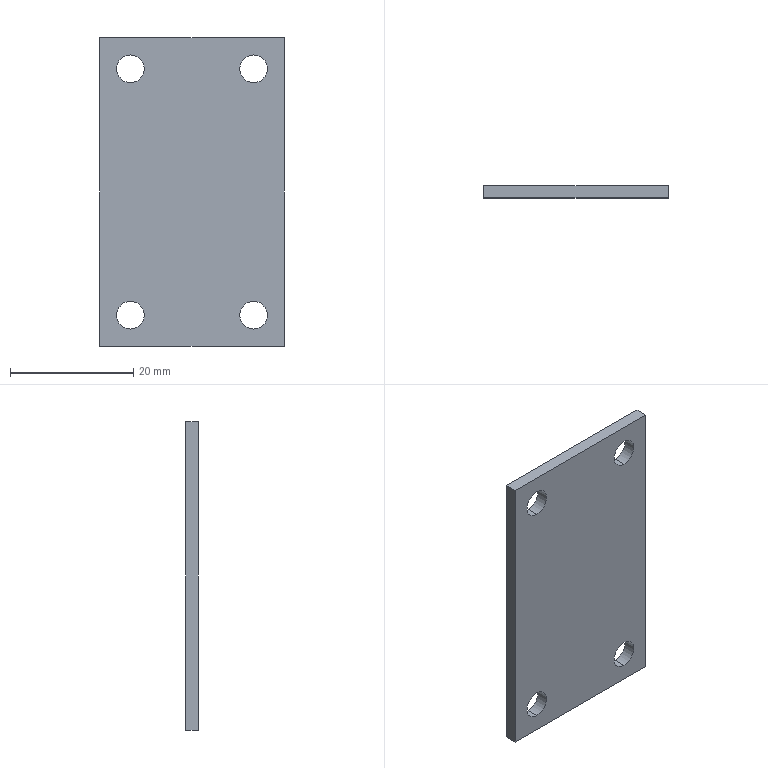Part | STEP file | 0243_204_Push_Plate | 1 solid | 14 faces | box 30 x 2 x 50 mm | volume 2873 mm3 | cylinder 8 | plane 6 | commonest cylinder face diameters 4.5 x8
STEP:
#1=CARTESIAN_POINT('',(0.,0.,0.));
#2=DIRECTION('',(0.,0.,1.));
#3=DIRECTION('',(1.,0.,0.));
#4=AXIS2_PLACEMENT_3D('',#1,#2,#3);
#5=CARTESIAN_POINT('',(-25.,0.,22.25));
#6=VERTEX_POINT('',#5);
#7=CARTESIAN_POINT('',(-25.,2.,22.25));
#8=VERTEX_POINT('',#7);
#9=CARTESIAN_POINT('',(-25.,2.,22.25));
#10=DIRECTION('',(0.,1.,0.));
#11=VECTOR('',#10,1.);
#12=LINE('',#9,#11);
#13=CARTESIAN_POINT('',(-25.,2.,20.));
#14=DIRECTION('',(0.,1.,0.));
#15=DIRECTION('',(0.,0.,1.));
#16=AXIS2_PLACEMENT_3D('',#13,#14,#15);
#17=CYLINDRICAL_SURFACE('',#16,2.25);
#18=CARTESIAN_POINT('',(6.283,0.));
#19=DIRECTION('',(0.,1.));
#20=VECTOR('',#19,1.);
#21=LINE('',#18,#20);
#22=(GEOMETRIC_REPRESENTATION_CONTEXT(2)PARAMETRIC_REPRESENTATION_CONTEXT()REPRESENTATION_CONTEXT('',''));
#23=DEFINITIONAL_REPRESENTATION('',(#21),#22);
#24=PCURVE('',#17,#23);
#25=CARTESIAN_POINT('',(-25.,2.,20.));
#26=DIRECTION('',(0.,1.,0.));
#27=DIRECTION('',(0.,0.,1.));
#28=AXIS2_PLACEMENT_3D('',#25,#26,#27);
#29=CYLINDRICAL_SURFACE('',#28,2.25);
#30=CARTESIAN_POINT('',(0.,0.));
#31=DIRECTION('',(0.,1.));
#32=VECTOR('',#31,1.);
#33=LINE('',#30,#32);
#34=(GEOMETRIC_REPRESENTATION_CONTEXT(2)PARAMETRIC_REPRESENTATION_CONTEXT()REPRESENTATION_CONTEXT('',''));
#35=DEFINITIONAL_REPRESENTATION('',(#33),#34);
#36=PCURVE('',#29,#35);
#37=SURFACE_CURVE('',#12,(#24,#36),.PCURVE_S1.);
#38=EDGE_CURVE('',#6,#8,#37,.T.);
#39=ORIENTED_EDGE('',*,*,#38,.T.);
#40=CARTESIAN_POINT('',(-25.,2.,17.75));
#41=VERTEX_POINT('',#40);
#42=CARTESIAN_POINT('',(-25.,2.,20.));
#43=DIRECTION('',(0.,1.,0.));
#44=DIRECTION('',(0.,0.,1.));
#45=AXIS2_PLACEMENT_3D('',#42,#43,#44);
#46=CIRCLE('',#45,2.25);
#47=CARTESIAN_POINT('',(0.,0.));
#48=DIRECTION('',(1.,0.));
#49=VECTOR('',#48,1.);
#50=LINE('',#47,#49);
#51=(GEOMETRIC_REPRESENTATION_CONTEXT(2)PARAMETRIC_REPRESENTATION_CONTEXT()REPRESENTATION_CONTEXT('',''));
#52=DEFINITIONAL_REPRESENTATION('',(#50),#51);
#53=PCURVE('',#17,#52);
#54=CARTESIAN_POINT('',(-30.,2.,25.));
#55=DIRECTION('',(0.,-1.,0.));
#56=DIRECTION('',(0.,0.,-1.));
#57=AXIS2_PLACEMENT_3D('',#54,#55,#56);
#58=PLANE('',#57);
#59=CARTESIAN_POINT('',(2.75,5.));
#60=CARTESIAN_POINT('',(2.75,8.897));
#61=CARTESIAN_POINT('',(6.125,6.949));
#62=CARTESIAN_POINT('',(9.5,5.));
#63=CARTESIAN_POINT('',(6.125,3.051));
#64=CARTESIAN_POINT('',(2.75,1.103));
#65=CARTESIAN_POINT('',(2.75,5.));
#66=(BOUNDED_CURVE()B_SPLINE_CURVE(2,(#59,#60,#61,#62,#63,#64,#65),.UNSPECIFIED.,.T.,.F.)B_SPLINE_CURVE_WITH_KNOTS((1,2,2,2,2,1),(-2.094,0.,2.094,4.189,6.283,8.378),.UNSPECIFIED.)CURVE()GEOMETRIC_REPRESENTATION_ITEM()RATIONAL_B_SPLINE_CURVE((1.,0.5,1.,0.5,1.,0.5,1.))REPRESENTATION_ITEM(''));
#67=(GEOMETRIC_REPRESENTATION_CONTEXT(2)PARAMETRIC_REPRESENTATION_CONTEXT()REPRESENTATION_CONTEXT('',''));
#68=DEFINITIONAL_REPRESENTATION('',(#66),#67);
#69=PCURVE('',#58,#68);
#70=SURFACE_CURVE('',#46,(#53,#69),.PCURVE_S1.);
#71=EDGE_CURVE('',#41,#8,#70,.T.);
#72=ORIENTED_EDGE('',*,*,#71,.F.);
#73=CARTESIAN_POINT('',(-25.,0.,17.75));
#74=VERTEX_POINT('',#73);
#75=CARTESIAN_POINT('',(-25.,2.,17.75));
#76=DIRECTION('',(0.,1.,0.));
#77=VECTOR('',#76,1.);
#78=LINE('',#75,#77);
#79=CARTESIAN_POINT('',(3.142,0.));
#80=DIRECTION('',(0.,1.));
#81=VECTOR('',#80,1.);
#82=LINE('',#79,#81);
#83=(GEOMETRIC_REPRESENTATION_CONTEXT(2)PARAMETRIC_REPRESENTATION_CONTEXT()REPRESENTATION_CONTEXT('',''));
#84=DEFINITIONAL_REPRESENTATION('',(#82),#83);
#85=PCURVE('',#17,#84);
#86=CARTESIAN_POINT('',(3.142,0.));
#87=DIRECTION('',(0.,1.));
#88=VECTOR('',#87,1.);
#89=LINE('',#86,#88);
#90=(GEOMETRIC_REPRESENTATION_CONTEXT(2)PARAMETRIC_REPRESENTATION_CONTEXT()REPRESENTATION_CONTEXT('',''));
#91=DEFINITIONAL_REPRESENTATION('',(#89),#90);
#92=PCURVE('',#29,#91);
#93=SURFACE_CURVE('',#78,(#85,#92),.PCURVE_S1.);
#94=EDGE_CURVE('',#74,#41,#93,.T.);
#95=ORIENTED_EDGE('',*,*,#94,.F.);
#96=CARTESIAN_POINT('',(-25.,0.,20.));
#97=DIRECTION('',(0.,1.,0.));
#98=DIRECTION('',(0.,0.,1.));
#99=AXIS2_PLACEMENT_3D('',#96,#97,#98);
#100=CIRCLE('',#99,2.25);
#101=CARTESIAN_POINT('',(0.,-2.));
#102=DIRECTION('',(1.,0.));
#103=VECTOR('',#102,1.);
#104=LINE('',#101,#103);
#105=(GEOMETRIC_REPRESENTATION_CONTEXT(2)PARAMETRIC_REPRESENTATION_CONTEXT()REPRESENTATION_CONTEXT('',''));
#106=DEFINITIONAL_REPRESENTATION('',(#104),#105);
#107=PCURVE('',#17,#106);
#108=CARTESIAN_POINT('',(-30.,0.,25.));
#109=DIRECTION('',(0.,-1.,0.));
#110=DIRECTION('',(0.,0.,-1.));
#111=AXIS2_PLACEMENT_3D('',#108,#109,#110);
#112=PLANE('',#111);
#113=CARTESIAN_POINT('',(2.75,5.));
#114=CARTESIAN_POINT('',(2.75,8.897));
#115=CARTESIAN_POINT('',(6.125,6.949));
#116=CARTESIAN_POINT('',(9.5,5.));
#117=CARTESIAN_POINT('',(6.125,3.051));
#118=CARTESIAN_POINT('',(2.75,1.103));
#119=CARTESIAN_POINT('',(2.75,5.));
#120=(BOUNDED_CURVE()B_SPLINE_CURVE(2,(#113,#114,#115,#116,#117,#118,#119),.UNSPECIFIED.,.T.,.F.)B_SPLINE_CURVE_WITH_KNOTS((1,2,2,2,2,1),(-2.094,0.,2.094,4.189,6.283,8.378),.UNSPECIFIED.)CURVE()GEOMETRIC_REPRESENTATION_ITEM()RATIONAL_B_SPLINE_CURVE((1.,0.5,1.,0.5,1.,0.5,1.))REPRESENTATION_ITEM(''));
#121=(GEOMETRIC_REPRESENTATION_CONTEXT(2)PARAMETRIC_REPRESENTATION_CONTEXT()REPRESENTATION_CONTEXT('',''));
#122=DEFINITIONAL_REPRESENTATION('',(#120),#121);
#123=PCURVE('',#112,#122);
#124=SURFACE_CURVE('',#100,(#107,#123),.PCURVE_S1.);
#125=EDGE_CURVE('',#74,#6,#124,.T.);
#126=ORIENTED_EDGE('',*,*,#125,.T.);
#127=EDGE_LOOP('',(#39,#72,#95,#126));
#128=FACE_BOUND('',#127,.F.);
#129=ADVANCED_FACE('',(#128),#17,.F.);
#130=CARTESIAN_POINT('',(-25.,0.,-17.75));
#131=VERTEX_POINT('',#130);
#132=CARTESIAN_POINT('',(-25.,2.,-17.75));
#133=VERTEX_POINT('',#132);
#134=CARTESIAN_POINT('',(-25.,2.,-17.75));
#135=DIRECTION('',(0.,1.,0.));
#136=VECTOR('',#135,1.);
#137=LINE('',#134,#136);
#138=CARTESIAN_POINT('',(-25.,2.,-20.));
#139=DIRECTION('',(0.,1.,0.));
#140=DIRECTION('',(0.,0.,1.));
#141=AXIS2_PLACEMENT_3D('',#138,#139,#140);
#142=CYLINDRICAL_SURFACE('',#141,2.25);
#143=CARTESIAN_POINT('',(6.283,0.));
#144=DIRECTION('',(0.,1.));
#145=VECTOR('',#144,1.);
#146=LINE('',#143,#145);
#147=(GEOMETRIC_REPRESENTATION_CONTEXT(2)PARAMETRIC_REPRESENTATION_CONTEXT()REPRESENTATION_CONTEXT('',''));
#148=DEFINITIONAL_REPRESENTATION('',(#146),#147);
#149=PCURVE('',#142,#148);
#150=CARTESIAN_POINT('',(-25.,2.,-20.));
#151=DIRECTION('',(0.,1.,0.));
#152=DIRECTION('',(0.,0.,1.));
#153=AXIS2_PLACEMENT_3D('',#150,#151,#152);
#154=CYLINDRICAL_SURFACE('',#153,2.25);
#155=CARTESIAN_POINT('',(0.,0.));
#156=DIRECTION('',(0.,1.));
#157=VECTOR('',#156,1.);
#158=LINE('',#155,#157);
#159=(GEOMETRIC_REPRESENTATION_CONTEXT(2)PARAMETRIC_REPRESENTATION_CONTEXT()REPRESENTATION_CONTEXT('',''));
#160=DEFINITIONAL_REPRESENTATION('',(#158),#159);
#161=PCURVE('',#154,#160);
#162=SURFACE_CURVE('',#137,(#149,#161),.PCURVE_S1.);
#163=EDGE_CURVE('',#131,#133,#162,.T.);
#164=ORIENTED_EDGE('',*,*,#163,.T.);
#165=CARTESIAN_POINT('',(-25.,2.,-22.25));
#166=VERTEX_POINT('',#165);
#167=CARTESIAN_POINT('',(-25.,2.,-20.));
#168=DIRECTION('',(0.,1.,0.));
#169=DIRECTION('',(0.,0.,1.));
#170=AXIS2_PLACEMENT_3D('',#167,#168,#169);
#171=CIRCLE('',#170,2.25);
#172=CARTESIAN_POINT('',(0.,0.));
#173=DIRECTION('',(1.,0.));
#174=VECTOR('',#173,1.);
#175=LINE('',#172,#174);
#176=(GEOMETRIC_REPRESENTATION_CONTEXT(2)PARAMETRIC_REPRESENTATION_CONTEXT()REPRESENTATION_CONTEXT('',''));
#177=DEFINITIONAL_REPRESENTATION('',(#175),#176);
#178=PCURVE('',#142,#177);
#179=CARTESIAN_POINT('',(42.75,5.));
#180=CARTESIAN_POINT('',(42.75,8.897));
#181=CARTESIAN_POINT('',(46.125,6.949));
#182=CARTESIAN_POINT('',(49.5,5.));
#183=CARTESIAN_POINT('',(46.125,3.051));
#184=CARTESIAN_POINT('',(42.75,1.103));
#185=CARTESIAN_POINT('',(42.75,5.));
#186=(BOUNDED_CURVE()B_SPLINE_CURVE(2,(#179,#180,#181,#182,#183,#184,#185),.UNSPECIFIED.,.T.,.F.)B_SPLINE_CURVE_WITH_KNOTS((1,2,2,2,2,1),(-2.094,0.,2.094,4.189,6.283,8.378),.UNSPECIFIED.)CURVE()GEOMETRIC_REPRESENTATION_ITEM()RATIONAL_B_SPLINE_CURVE((1.,0.5,1.,0.5,1.,0.5,1.))REPRESENTATION_ITEM(''));
#187=(GEOMETRIC_REPRESENTATION_CONTEXT(2)PARAMETRIC_REPRESENTATION_CONTEXT()REPRESENTATION_CONTEXT('',''));
#188=DEFINITIONAL_REPRESENTATION('',(#186),#187);
#189=PCURVE('',#58,#188);
#190=SURFACE_CURVE('',#171,(#178,#189),.PCURVE_S1.);
#191=EDGE_CURVE('',#166,#133,#190,.T.);
#192=ORIENTED_EDGE('',*,*,#191,.F.);
#193=CARTESIAN_POINT('',(-25.,0.,-22.25));
#194=VERTEX_POINT('',#193);
#195=CARTESIAN_POINT('',(-25.,2.,-22.25));
#196=DIRECTION('',(0.,1.,0.));
#197=VECTOR('',#196,1.);
#198=LINE('',#195,#197);
#199=CARTESIAN_POINT('',(3.142,0.));
#200=DIRECTION('',(0.,1.));
#201=VECTOR('',#200,1.);
#202=LINE('',#199,#201);
#203=(GEOMETRIC_REPRESENTATION_CONTEXT(2)PARAMETRIC_REPRESENTATION_CONTEXT()REPRESENTATION_CONTEXT('',''));
#204=DEFINITIONAL_REPRESENTATION('',(#202),#203);
#205=PCURVE('',#142,#204);
#206=CARTESIAN_POINT('',(3.142,0.));
#207=DIRECTION('',(0.,1.));
#208=VECTOR('',#207,1.);
#209=LINE('',#206,#208);
#210=(GEOMETRIC_REPRESENTATION_CONTEXT(2)PARAMETRIC_REPRESENTATION_CONTEXT()REPRESENTATION_CONTEXT('',''));
#211=DEFINITIONAL_REPRESENTATION('',(#209),#210);
#212=PCURVE('',#154,#211);
#213=SURFACE_CURVE('',#198,(#205,#212),.PCURVE_S1.);
#214=EDGE_CURVE('',#194,#166,#213,.T.);
#215=ORIENTED_EDGE('',*,*,#214,.F.);
#216=CARTESIAN_POINT('',(-25.,0.,-20.));
#217=DIRECTION('',(0.,1.,0.));
#218=DIRECTION('',(0.,0.,1.));
#219=AXIS2_PLACEMENT_3D('',#216,#217,#218);
#220=CIRCLE('',#219,2.25);
#221=CARTESIAN_POINT('',(0.,-2.));
#222=DIRECTION('',(1.,0.));
#223=VECTOR('',#222,1.);
#224=LINE('',#221,#223);
#225=(GEOMETRIC_REPRESENTATION_CONTEXT(2)PARAMETRIC_REPRESENTATION_CONTEXT()REPRESENTATION_CONTEXT('',''));
#226=DEFINITIONAL_REPRESENTATION('',(#224),#225);
#227=PCURVE('',#142,#226);
#228=CARTESIAN_POINT('',(42.75,5.));
#229=CARTESIAN_POINT('',(42.75,8.897));
#230=CARTESIAN_POINT('',(46.125,6.949));
#231=CARTESIAN_POINT('',(49.5,5.));
#232=CARTESIAN_POINT('',(46.125,3.051));
#233=CARTESIAN_POINT('',(42.75,1.103));
#234=CARTESIAN_POINT('',(42.75,5.));
#235=(BOUNDED_CURVE()B_SPLINE_CURVE(2,(#228,#229,#230,#231,#232,#233,#234),.UNSPECIFIED.,.T.,.F.)B_SPLINE_CURVE_WITH_KNOTS((1,2,2,2,2,1),(-2.094,0.,2.094,4.189,6.283,8.378),.UNSPECIFIED.)CURVE()GEOMETRIC_REPRESENTATION_ITEM()RATIONAL_B_SPLINE_CURVE((1.,0.5,1.,0.5,1.,0.5,1.))REPRESENTATION_ITEM(''));
#236=(GEOMETRIC_REPRESENTATION_CONTEXT(2)PARAMETRIC_REPRESENTATION_CONTEXT()REPRESENTATION_CONTEXT('',''));
#237=DEFINITIONAL_REPRESENTATION('',(#235),#236);
#238=PCURVE('',#112,#237);
#239=SURFACE_CURVE('',#220,(#227,#238),.PCURVE_S1.);
#240=EDGE_CURVE('',#194,#131,#239,.T.);
#241=ORIENTED_EDGE('',*,*,#240,.T.);
#242=EDGE_LOOP('',(#164,#192,#215,#241));
#243=FACE_BOUND('',#242,.F.);
#244=ADVANCED_FACE('',(#243),#142,.F.);
#245=CARTESIAN_POINT('',(-5.,0.,-17.75));
#246=VERTEX_POINT('',#245);
#247=CARTESIAN_POINT('',(-5.,2.,-17.75));
#248=VERTEX_POINT('',#247);
#249=CARTESIAN_POINT('',(-5.,2.,-17.75));
#250=DIRECTION('',(0.,1.,0.));
#251=VECTOR('',#250,1.);
#252=LINE('',#249,#251);
#253=CARTESIAN_POINT('',(-5.,2.,-20.));
#254=DIRECTION('',(0.,1.,0.));
#255=DIRECTION('',(0.,0.,1.));
#256=AXIS2_PLACEMENT_3D('',#253,#254,#255);
#257=CYLINDRICAL_SURFACE('',#256,2.25);
#258=CARTESIAN_POINT('',(6.283,0.));
#259=DIRECTION('',(0.,1.));
#260=VECTOR('',#259,1.);
#261=LINE('',#258,#260);
#262=(GEOMETRIC_REPRESENTATION_CONTEXT(2)PARAMETRIC_REPRESENTATION_CONTEXT()REPRESENTATION_CONTEXT('',''));
#263=DEFINITIONAL_REPRESENTATION('',(#261),#262);
#264=PCURVE('',#257,#263);
#265=CARTESIAN_POINT('',(-5.,2.,-20.));
#266=DIRECTION('',(0.,1.,0.));
#267=DIRECTION('',(0.,0.,1.));
#268=AXIS2_PLACEMENT_3D('',#265,#266,#267);
#269=CYLINDRICAL_SURFACE('',#268,2.25);
#270=CARTESIAN_POINT('',(0.,0.));
#271=DIRECTION('',(0.,1.));
#272=VECTOR('',#271,1.);
#273=LINE('',#270,#272);
#274=(GEOMETRIC_REPRESENTATION_CONTEXT(2)PARAMETRIC_REPRESENTATION_CONTEXT()REPRESENTATION_CONTEXT('',''));
#275=DEFINITIONAL_REPRESENTATION('',(#273),#274);
#276=PCURVE('',#269,#275);
#277=SURFACE_CURVE('',#252,(#264,#276),.PCURVE_S1.);
#278=EDGE_CURVE('',#246,#248,#277,.T.);
#279=ORIENTED_EDGE('',*,*,#278,.T.);
#280=CARTESIAN_POINT('',(-5.,2.,-22.25));
#281=VERTEX_POINT('',#280);
#282=CARTESIAN_POINT('',(-5.,2.,-20.));
#283=DIRECTION('',(0.,1.,0.));
#284=DIRECTION('',(0.,0.,1.));
#285=AXIS2_PLACEMENT_3D('',#282,#283,#284);
#286=CIRCLE('',#285,2.25);
#287=CARTESIAN_POINT('',(0.,0.));
#288=DIRECTION('',(1.,0.));
#289=VECTOR('',#288,1.);
#290=LINE('',#287,#289);
#291=(GEOMETRIC_REPRESENTATION_CONTEXT(2)PARAMETRIC_REPRESENTATION_CONTEXT()REPRESENTATION_CONTEXT('',''));
#292=DEFINITIONAL_REPRESENTATION('',(#290),#291);
#293=PCURVE('',#257,#292);
#294=CARTESIAN_POINT('',(42.75,25.));
#295=CARTESIAN_POINT('',(42.75,28.897));
#296=CARTESIAN_POINT('',(46.125,26.949));
#297=CARTESIAN_POINT('',(49.5,25.));
#298=CARTESIAN_POINT('',(46.125,23.051));
#299=CARTESIAN_POINT('',(42.75,21.103));
#300=CARTESIAN_POINT('',(42.75,25.));
#301=(BOUNDED_CURVE()B_SPLINE_CURVE(2,(#294,#295,#296,#297,#298,#299,#300),.UNSPECIFIED.,.T.,.F.)B_SPLINE_CURVE_WITH_KNOTS((1,2,2,2,2,1),(-2.094,0.,2.094,4.189,6.283,8.378),.UNSPECIFIED.)CURVE()GEOMETRIC_REPRESENTATION_ITEM()RATIONAL_B_SPLINE_CURVE((1.,0.5,1.,0.5,1.,0.5,1.))REPRESENTATION_ITEM(''));
#302=(GEOMETRIC_REPRESENTATION_CONTEXT(2)PARAMETRIC_REPRESENTATION_CONTEXT()REPRESENTATION_CONTEXT('',''));
#303=DEFINITIONAL_REPRESENTATION('',(#301),#302);
#304=PCURVE('',#58,#303);
#305=SURFACE_CURVE('',#286,(#293,#304),.PCURVE_S1.);
#306=EDGE_CURVE('',#281,#248,#305,.T.);
#307=ORIENTED_EDGE('',*,*,#306,.F.);
#308=CARTESIAN_POINT('',(-5.,0.,-22.25));
#309=VERTEX_POINT('',#308);
#310=CARTESIAN_POINT('',(-5.,2.,-22.25));
#311=DIRECTION('',(0.,1.,0.));
#312=VECTOR('',#311,1.);
#313=LINE('',#310,#312);
#314=CARTESIAN_POINT('',(3.142,0.));
#315=DIRECTION('',(0.,1.));
#316=VECTOR('',#315,1.);
#317=LINE('',#314,#316);
#318=(GEOMETRIC_REPRESENTATION_CONTEXT(2)PARAMETRIC_REPRESENTATION_CONTEXT()REPRESENTATION_CONTEXT('',''));
#319=DEFINITIONAL_REPRESENTATION('',(#317),#318);
#320=PCURVE('',#257,#319);
#321=CARTESIAN_POINT('',(3.142,0.));
#322=DIRECTION('',(0.,1.));
#323=VECTOR('',#322,1.);
#324=LINE('',#321,#323);
#325=(GEOMETRIC_REPRESENTATION_CONTEXT(2)PARAMETRIC_REPRESENTATION_CONTEXT()REPRESENTATION_CONTEXT('',''));
#326=DEFINITIONAL_REPRESENTATION('',(#324),#325);
#327=PCURVE('',#269,#326);
#328=SURFACE_CURVE('',#313,(#320,#327),.PCURVE_S1.);
#329=EDGE_CURVE('',#309,#281,#328,.T.);
#330=ORIENTED_EDGE('',*,*,#329,.F.);
#331=CARTESIAN_POINT('',(-5.,0.,-20.));
#332=DIRECTION('',(0.,1.,0.));
#333=DIRECTION('',(0.,0.,1.));
#334=AXIS2_PLACEMENT_3D('',#331,#332,#333);
#335=CIRCLE('',#334,2.25);
#336=CARTESIAN_POINT('',(0.,-2.));
#337=DIRECTION('',(1.,0.));
#338=VECTOR('',#337,1.);
#339=LINE('',#336,#338);
#340=(GEOMETRIC_REPRESENTATION_CONTEXT(2)PARAMETRIC_REPRESENTATION_CONTEXT()REPRESENTATION_CONTEXT('',''));
#341=DEFINITIONAL_REPRESENTATION('',(#339),#340);
#342=PCURVE('',#257,#341);
#343=CARTESIAN_POINT('',(42.75,25.));
#344=CARTESIAN_POINT('',(42.75,28.897));
#345=CARTESIAN_POINT('',(46.125,26.949));
#346=CARTESIAN_POINT('',(49.5,25.));
#347=CARTESIAN_POINT('',(46.125,23.051));
#348=CARTESIAN_POINT('',(42.75,21.103));
#349=CARTESIAN_POINT('',(42.75,25.));
#350=(BOUNDED_CURVE()B_SPLINE_CURVE(2,(#343,#344,#345,#346,#347,#348,#349),.UNSPECIFIED.,.T.,.F.)B_SPLINE_CURVE_WITH_KNOTS((1,2,2,2,2,1),(-2.094,0.,2.094,4.189,6.283,8.378),.UNSPECIFIED.)CURVE()GEOMETRIC_REPRESENTATION_ITEM()RATIONAL_B_SPLINE_CURVE((1.,0.5,1.,0.5,1.,0.5,1.))REPRESENTATION_ITEM(''));
#351=(GEOMETRIC_REPRESENTATION_CONTEXT(2)PARAMETRIC_REPRESENTATION_CONTEXT()REPRESENTATION_CONTEXT('',''));
#352=DEFINITIONAL_REPRESENTATION('',(#350),#351);
#353=PCURVE('',#112,#352);
#354=SURFACE_CURVE('',#335,(#342,#353),.PCURVE_S1.);
#355=EDGE_CURVE('',#309,#246,#354,.T.);
#356=ORIENTED_EDGE('',*,*,#355,.T.);
#357=EDGE_LOOP('',(#279,#307,#330,#356));
#358=FACE_BOUND('',#357,.F.);
#359=ADVANCED_FACE('',(#358),#257,.F.);
#360=CARTESIAN_POINT('',(-5.,0.,22.25));
#361=VERTEX_POINT('',#360);
#362=CARTESIAN_POINT('',(-5.,2.,22.25));
#363=VERTEX_POINT('',#362);
#364=CARTESIAN_POINT('',(-5.,2.,22.25));
#365=DIRECTION('',(0.,1.,0.));
#366=VECTOR('',#365,1.);
#367=LINE('',#364,#366);
#368=CARTESIAN_POINT('',(-5.,2.,20.));
#369=DIRECTION('',(0.,1.,0.));
#370=DIRECTION('',(0.,0.,1.));
#371=AXIS2_PLACEMENT_3D('',#368,#369,#370);
#372=CYLINDRICAL_SURFACE('',#371,2.25);
#373=CARTESIAN_POINT('',(6.283,0.));
#374=DIRECTION('',(0.,1.));
#375=VECTOR('',#374,1.);
#376=LINE('',#373,#375);
#377=(GEOMETRIC_REPRESENTATION_CONTEXT(2)PARAMETRIC_REPRESENTATION_CONTEXT()REPRESENTATION_CONTEXT('',''));
#378=DEFINITIONAL_REPRESENTATION('',(#376),#377);
#379=PCURVE('',#372,#378);
#380=CARTESIAN_POINT('',(-5.,2.,20.));
#381=DIRECTION('',(0.,1.,0.));
#382=DIRECTION('',(0.,0.,1.));
#383=AXIS2_PLACEMENT_3D('',#380,#381,#382);
#384=CYLINDRICAL_SURFACE('',#383,2.25);
#385=CARTESIAN_POINT('',(0.,0.));
#386=DIRECTION('',(0.,1.));
#387=VECTOR('',#386,1.);
#388=LINE('',#385,#387);
#389=(GEOMETRIC_REPRESENTATION_CONTEXT(2)PARAMETRIC_REPRESENTATION_CONTEXT()REPRESENTATION_CONTEXT('',''));
#390=DEFINITIONAL_REPRESENTATION('',(#388),#389);
#391=PCURVE('',#384,#390);
#392=SURFACE_CURVE('',#367,(#379,#391),.PCURVE_S1.);
#393=EDGE_CURVE('',#361,#363,#392,.T.);
#394=ORIENTED_EDGE('',*,*,#393,.T.);
#395=CARTESIAN_POINT('',(-5.,2.,17.75));
#396=VERTEX_POINT('',#395);
#397=CARTESIAN_POINT('',(-5.,2.,20.));
#398=DIRECTION('',(0.,1.,0.));
#399=DIRECTION('',(0.,0.,1.));
#400=AXIS2_PLACEMENT_3D('',#397,#398,#399);
#401=CIRCLE('',#400,2.25);
#402=CARTESIAN_POINT('',(0.,0.));
#403=DIRECTION('',(1.,0.));
#404=VECTOR('',#403,1.);
#405=LINE('',#402,#404);
#406=(GEOMETRIC_REPRESENTATION_CONTEXT(2)PARAMETRIC_REPRESENTATION_CONTEXT()REPRESENTATION_CONTEXT('',''));
#407=DEFINITIONAL_REPRESENTATION('',(#405),#406);
#408=PCURVE('',#372,#407);
#409=CARTESIAN_POINT('',(2.75,25.));
#410=CARTESIAN_POINT('',(2.75,28.897));
#411=CARTESIAN_POINT('',(6.125,26.949));
#412=CARTESIAN_POINT('',(9.5,25.));
#413=CARTESIAN_POINT('',(6.125,23.051));
#414=CARTESIAN_POINT('',(2.75,21.103));
#415=CARTESIAN_POINT('',(2.75,25.));
#416=(BOUNDED_CURVE()B_SPLINE_CURVE(2,(#409,#410,#411,#412,#413,#414,#415),.UNSPECIFIED.,.T.,.F.)B_SPLINE_CURVE_WITH_KNOTS((1,2,2,2,2,1),(-2.094,0.,2.094,4.189,6.283,8.378),.UNSPECIFIED.)CURVE()GEOMETRIC_REPRESENTATION_ITEM()RATIONAL_B_SPLINE_CURVE((1.,0.5,1.,0.5,1.,0.5,1.))REPRESENTATION_ITEM(''));
#417=(GEOMETRIC_REPRESENTATION_CONTEXT(2)PARAMETRIC_REPRESENTATION_CONTEXT()REPRESENTATION_CONTEXT('',''));
#418=DEFINITIONAL_REPRESENTATION('',(#416),#417);
#419=PCURVE('',#58,#418);
#420=SURFACE_CURVE('',#401,(#408,#419),.PCURVE_S1.);
#421=EDGE_CURVE('',#396,#363,#420,.T.);
#422=ORIENTED_EDGE('',*,*,#421,.F.);
#423=CARTESIAN_POINT('',(-5.,0.,17.75));
#424=VERTEX_POINT('',#423);
#425=CARTESIAN_POINT('',(-5.,2.,17.75));
#426=DIRECTION('',(0.,1.,0.));
#427=VECTOR('',#426,1.);
#428=LINE('',#425,#427);
#429=CARTESIAN_POINT('',(3.142,0.));
#430=DIRECTION('',(0.,1.));
#431=VECTOR('',#430,1.);
#432=LINE('',#429,#431);
#433=(GEOMETRIC_REPRESENTATION_CONTEXT(2)PARAMETRIC_REPRESENTATION_CONTEXT()REPRESENTATION_CONTEXT('',''));
#434=DEFINITIONAL_REPRESENTATION('',(#432),#433);
#435=PCURVE('',#372,#434);
#436=CARTESIAN_POINT('',(3.142,0.));
#437=DIRECTION('',(0.,1.));
#438=VECTOR('',#437,1.);
#439=LINE('',#436,#438);
#440=(GEOMETRIC_REPRESENTATION_CONTEXT(2)PARAMETRIC_REPRESENTATION_CONTEXT()REPRESENTATION_CONTEXT('',''));
#441=DEFINITIONAL_REPRESENTATION('',(#439),#440);
#442=PCURVE('',#384,#441);
#443=SURFACE_CURVE('',#428,(#435,#442),.PCURVE_S1.);
#444=EDGE_CURVE('',#424,#396,#443,.T.);
#445=ORIENTED_EDGE('',*,*,#444,.F.);
#446=CARTESIAN_POINT('',(-5.,0.,20.));
#447=DIRECTION('',(0.,1.,0.));
#448=DIRECTION('',(0.,0.,1.));
#449=AXIS2_PLACEMENT_3D('',#446,#447,#448);
#450=CIRCLE('',#449,2.25);
#451=CARTESIAN_POINT('',(0.,-2.));
#452=DIRECTION('',(1.,0.));
#453=VECTOR('',#452,1.);
#454=LINE('',#451,#453);
#455=(GEOMETRIC_REPRESENTATION_CONTEXT(2)PARAMETRIC_REPRESENTATION_CONTEXT()REPRESENTATION_CONTEXT('',''));
#456=DEFINITIONAL_REPRESENTATION('',(#454),#455);
#457=PCURVE('',#372,#456);
#458=CARTESIAN_POINT('',(2.75,25.));
#459=CARTESIAN_POINT('',(2.75,28.897));
#460=CARTESIAN_POINT('',(6.125,26.949));
#461=CARTESIAN_POINT('',(9.5,25.));
#462=CARTESIAN_POINT('',(6.125,23.051));
#463=CARTESIAN_POINT('',(2.75,21.103));
#464=CARTESIAN_POINT('',(2.75,25.));
#465=(BOUNDED_CURVE()B_SPLINE_CURVE(2,(#458,#459,#460,#461,#462,#463,#464),.UNSPECIFIED.,.T.,.F.)B_SPLINE_CURVE_WITH_KNOTS((1,2,2,2,2,1),(-2.094,0.,2.094,4.189,6.283,8.378),.UNSPECIFIED.)CURVE()GEOMETRIC_REPRESENTATION_ITEM()RATIONAL_B_SPLINE_CURVE((1.,0.5,1.,0.5,1.,0.5,1.))REPRESENTATION_ITEM(''));
#466=(GEOMETRIC_REPRESENTATION_CONTEXT(2)PARAMETRIC_REPRESENTATION_CONTEXT()REPRESENTATION_CONTEXT('',''));
#467=DEFINITIONAL_REPRESENTATION('',(#465),#466);
#468=PCURVE('',#112,#467);
#469=SURFACE_CURVE('',#450,(#457,#468),.PCURVE_S1.);
#470=EDGE_CURVE('',#424,#361,#469,.T.);
#471=ORIENTED_EDGE('',*,*,#470,.T.);
#472=EDGE_LOOP('',(#394,#422,#445,#471));
#473=FACE_BOUND('',#472,.F.);
#474=ADVANCED_FACE('',(#473),#372,.F.);
#475=CARTESIAN_POINT('',(-30.,0.,25.));
#476=VERTEX_POINT('',#475);
#477=CARTESIAN_POINT('',(0.,0.,25.));
#478=VERTEX_POINT('',#477);
#479=CARTESIAN_POINT('',(0.,0.,25.));
#480=DIRECTION('',(1.,0.,0.));
#481=VECTOR('',#480,1.);
#482=LINE('',#479,#481);
#483=CARTESIAN_POINT('',(0.,2.,25.));
#484=DIRECTION('',(0.,0.,-1.));
#485=DIRECTION('',(-1.,0.,0.));
#486=AXIS2_PLACEMENT_3D('',#483,#484,#485);
#487=PLANE('',#486);
#488=CARTESIAN_POINT('',(0.,-2.));
#489=DIRECTION('',(-1.,0.));
#490=VECTOR('',#489,1.);
#491=LINE('',#488,#490);
#492=(GEOMETRIC_REPRESENTATION_CONTEXT(2)PARAMETRIC_REPRESENTATION_CONTEXT()REPRESENTATION_CONTEXT('',''));
#493=DEFINITIONAL_REPRESENTATION('',(#491),#492);
#494=PCURVE('',#487,#493);
#495=CARTESIAN_POINT('',(0.,30.));
#496=DIRECTION('',(0.,1.));
#497=VECTOR('',#496,1.);
#498=LINE('',#495,#497);
#499=(GEOMETRIC_REPRESENTATION_CONTEXT(2)PARAMETRIC_REPRESENTATION_CONTEXT()REPRESENTATION_CONTEXT('',''));
#500=DEFINITIONAL_REPRESENTATION('',(#498),#499);
#501=PCURVE('',#112,#500);
#502=SURFACE_CURVE('',#482,(#494,#501),.PCURVE_S1.);
#503=EDGE_CURVE('',#476,#478,#502,.T.);
#504=ORIENTED_EDGE('',*,*,#503,.T.);
#505=CARTESIAN_POINT('',(0.,2.,25.));
#506=VERTEX_POINT('',#505);
#507=CARTESIAN_POINT('',(0.,2.,25.));
#508=DIRECTION('',(0.,-1.,0.));
#509=VECTOR('',#508,1.);
#510=LINE('',#507,#509);
#511=CARTESIAN_POINT('',(0.,0.));
#512=DIRECTION('',(0.,-1.));
#513=VECTOR('',#512,1.);
#514=LINE('',#511,#513);
#515=(GEOMETRIC_REPRESENTATION_CONTEXT(2)PARAMETRIC_REPRESENTATION_CONTEXT()REPRESENTATION_CONTEXT('',''));
#516=DEFINITIONAL_REPRESENTATION('',(#514),#515);
#517=PCURVE('',#487,#516);
#518=CARTESIAN_POINT('',(0.,2.,25.));
#519=DIRECTION('',(-1.,0.,0.));
#520=DIRECTION('',(0.,0.,1.));
#521=AXIS2_PLACEMENT_3D('',#518,#519,#520);
#522=PLANE('',#521);
#523=CARTESIAN_POINT('',(0.,0.));
#524=DIRECTION('',(0.,-1.));
#525=VECTOR('',#524,1.);
#526=LINE('',#523,#525);
#527=(GEOMETRIC_REPRESENTATION_CONTEXT(2)PARAMETRIC_REPRESENTATION_CONTEXT()REPRESENTATION_CONTEXT('',''));
#528=DEFINITIONAL_REPRESENTATION('',(#526),#527);
#529=PCURVE('',#522,#528);
#530=SURFACE_CURVE('',#510,(#517,#529),.PCURVE_S1.);
#531=EDGE_CURVE('',#506,#478,#530,.T.);
#532=ORIENTED_EDGE('',*,*,#531,.F.);
#533=CARTESIAN_POINT('',(-30.,2.,25.));
#534=VERTEX_POINT('',#533);
#535=CARTESIAN_POINT('',(0.,2.,25.));
#536=DIRECTION('',(1.,0.,0.));
#537=VECTOR('',#536,1.);
#538=LINE('',#535,#537);
#539=CARTESIAN_POINT('',(0.,0.));
#540=DIRECTION('',(-1.,0.));
#541=VECTOR('',#540,1.);
#542=LINE('',#539,#541);
#543=(GEOMETRIC_REPRESENTATION_CONTEXT(2)PARAMETRIC_REPRESENTATION_CONTEXT()REPRESENTATION_CONTEXT('',''));
#544=DEFINITIONAL_REPRESENTATION('',(#542),#543);
#545=PCURVE('',#487,#544);
#546=CARTESIAN_POINT('',(0.,30.));
#547=DIRECTION('',(0.,1.));
#548=VECTOR('',#547,1.);
#549=LINE('',#546,#548);
#550=(GEOMETRIC_REPRESENTATION_CONTEXT(2)PARAMETRIC_REPRESENTATION_CONTEXT()REPRESENTATION_CONTEXT('',''));
#551=DEFINITIONAL_REPRESENTATION('',(#549),#550);
#552=PCURVE('',#58,#551);
#553=SURFACE_CURVE('',#538,(#545,#552),.PCURVE_S1.);
#554=EDGE_CURVE('',#534,#506,#553,.T.);
#555=ORIENTED_EDGE('',*,*,#554,.F.);
#556=CARTESIAN_POINT('',(-30.,2.,25.));
#557=DIRECTION('',(0.,-1.,0.));
#558=VECTOR('',#557,1.);
#559=LINE('',#556,#558);
#560=CARTESIAN_POINT('',(30.,0.));
#561=DIRECTION('',(0.,-1.));
#562=VECTOR('',#561,1.);
#563=LINE('',#560,#562);
#564=(GEOMETRIC_REPRESENTATION_CONTEXT(2)PARAMETRIC_REPRESENTATION_CONTEXT()REPRESENTATION_CONTEXT('',''));
#565=DEFINITIONAL_REPRESENTATION('',(#563),#564);
#566=PCURVE('',#487,#565);
#567=CARTESIAN_POINT('',(-30.,2.,25.));
#568=DIRECTION('',(1.,0.,0.));
#569=DIRECTION('',(0.,0.,-1.));
#570=AXIS2_PLACEMENT_3D('',#567,#568,#569);
#571=PLANE('',#570);
#572=CARTESIAN_POINT('',(0.,0.));
#573=DIRECTION('',(0.,-1.));
#574=VECTOR('',#573,1.);
#575=LINE('',#572,#574);
#576=(GEOMETRIC_REPRESENTATION_CONTEXT(2)PARAMETRIC_REPRESENTATION_CONTEXT()REPRESENTATION_CONTEXT('',''));
#577=DEFINITIONAL_REPRESENTATION('',(#575),#576);
#578=PCURVE('',#571,#577);
#579=SURFACE_CURVE('',#559,(#566,#578),.PCURVE_S1.);
#580=EDGE_CURVE('',#534,#476,#579,.T.);
#581=ORIENTED_EDGE('',*,*,#580,.T.);
#582=EDGE_LOOP('',(#504,#532,#555,#581));
#583=FACE_BOUND('',#582,.T.);
#584=ADVANCED_FACE('',(#583),#487,.F.);
#585=CARTESIAN_POINT('',(0.,0.,-25.));
#586=VERTEX_POINT('',#585);
#587=CARTESIAN_POINT('',(0.,0.,25.));
#588=DIRECTION('',(0.,0.,-1.));
#589=VECTOR('',#588,1.);
#590=LINE('',#587,#589);
#591=CARTESIAN_POINT('',(0.,-2.));
#592=DIRECTION('',(-1.,0.));
#593=VECTOR('',#592,1.);
#594=LINE('',#591,#593);
#595=(GEOMETRIC_REPRESENTATION_CONTEXT(2)PARAMETRIC_REPRESENTATION_CONTEXT()REPRESENTATION_CONTEXT('',''));
#596=DEFINITIONAL_REPRESENTATION('',(#594),#595);
#597=PCURVE('',#522,#596);
#598=CARTESIAN_POINT('',(0.,30.));
#599=DIRECTION('',(1.,0.));
#600=VECTOR('',#599,1.);
#601=LINE('',#598,#600);
#602=(GEOMETRIC_REPRESENTATION_CONTEXT(2)PARAMETRIC_REPRESENTATION_CONTEXT()REPRESENTATION_CONTEXT('',''));
#603=DEFINITIONAL_REPRESENTATION('',(#601),#602);
#604=PCURVE('',#112,#603);
#605=SURFACE_CURVE('',#590,(#597,#604),.PCURVE_S1.);
#606=EDGE_CURVE('',#478,#586,#605,.T.);
#607=ORIENTED_EDGE('',*,*,#606,.T.);
#608=CARTESIAN_POINT('',(0.,2.,-25.));
#609=VERTEX_POINT('',#608);
#610=CARTESIAN_POINT('',(0.,2.,-25.));
#611=DIRECTION('',(0.,-1.,0.));
#612=VECTOR('',#611,1.);
#613=LINE('',#610,#612);
#614=CARTESIAN_POINT('',(-50.,0.));
#615=DIRECTION('',(0.,-1.));
#616=VECTOR('',#615,1.);
#617=LINE('',#614,#616);
#618=(GEOMETRIC_REPRESENTATION_CONTEXT(2)PARAMETRIC_REPRESENTATION_CONTEXT()REPRESENTATION_CONTEXT('',''));
#619=DEFINITIONAL_REPRESENTATION('',(#617),#618);
#620=PCURVE('',#522,#619);
#621=CARTESIAN_POINT('',(0.,2.,-25.));
#622=DIRECTION('',(0.,0.,1.));
#623=DIRECTION('',(1.,0.,0.));
#624=AXIS2_PLACEMENT_3D('',#621,#622,#623);
#625=PLANE('',#624);
#626=CARTESIAN_POINT('',(0.,0.));
#627=DIRECTION('',(0.,-1.));
#628=VECTOR('',#627,1.);
#629=LINE('',#626,#628);
#630=(GEOMETRIC_REPRESENTATION_CONTEXT(2)PARAMETRIC_REPRESENTATION_CONTEXT()REPRESENTATION_CONTEXT('',''));
#631=DEFINITIONAL_REPRESENTATION('',(#629),#630);
#632=PCURVE('',#625,#631);
#633=SURFACE_CURVE('',#613,(#620,#632),.PCURVE_S1.);
#634=EDGE_CURVE('',#609,#586,#633,.T.);
#635=ORIENTED_EDGE('',*,*,#634,.F.);
#636=CARTESIAN_POINT('',(0.,2.,25.));
#637=DIRECTION('',(0.,0.,-1.));
#638=VECTOR('',#637,1.);
#639=LINE('',#636,#638);
#640=CARTESIAN_POINT('',(0.,0.));
#641=DIRECTION('',(-1.,0.));
#642=VECTOR('',#641,1.);
#643=LINE('',#640,#642);
#644=(GEOMETRIC_REPRESENTATION_CONTEXT(2)PARAMETRIC_REPRESENTATION_CONTEXT()REPRESENTATION_CONTEXT('',''));
#645=DEFINITIONAL_REPRESENTATION('',(#643),#644);
#646=PCURVE('',#522,#645);
#647=CARTESIAN_POINT('',(0.,30.));
#648=DIRECTION('',(1.,0.));
#649=VECTOR('',#648,1.);
#650=LINE('',#647,#649);
#651=(GEOMETRIC_REPRESENTATION_CONTEXT(2)PARAMETRIC_REPRESENTATION_CONTEXT()REPRESENTATION_CONTEXT('',''));
#652=DEFINITIONAL_REPRESENTATION('',(#650),#651);
#653=PCURVE('',#58,#652);
#654=SURFACE_CURVE('',#639,(#646,#653),.PCURVE_S1.);
#655=EDGE_CURVE('',#506,#609,#654,.T.);
#656=ORIENTED_EDGE('',*,*,#655,.F.);
#657=ORIENTED_EDGE('',*,*,#531,.T.);
#658=EDGE_LOOP('',(#607,#635,#656,#657));
#659=FACE_BOUND('',#658,.T.);
#660=ADVANCED_FACE('',(#659),#522,.F.);
#661=CARTESIAN_POINT('',(-30.,0.,-25.));
#662=VERTEX_POINT('',#661);
#663=CARTESIAN_POINT('',(0.,0.,-25.));
#664=DIRECTION('',(-1.,0.,0.));
#665=VECTOR('',#664,1.);
#666=LINE('',#663,#665);
#667=CARTESIAN_POINT('',(0.,-2.));
#668=DIRECTION('',(-1.,0.));
#669=VECTOR('',#668,1.);
#670=LINE('',#667,#669);
#671=(GEOMETRIC_REPRESENTATION_CONTEXT(2)PARAMETRIC_REPRESENTATION_CONTEXT()REPRESENTATION_CONTEXT('',''));
#672=DEFINITIONAL_REPRESENTATION('',(#670),#671);
#673=PCURVE('',#625,#672);
#674=CARTESIAN_POINT('',(50.,30.));
#675=DIRECTION('',(0.,-1.));
#676=VECTOR('',#675,1.);
#677=LINE('',#674,#676);
#678=(GEOMETRIC_REPRESENTATION_CONTEXT(2)PARAMETRIC_REPRESENTATION_CONTEXT()REPRESENTATION_CONTEXT('',''));
#679=DEFINITIONAL_REPRESENTATION('',(#677),#678);
#680=PCURVE('',#112,#679);
#681=SURFACE_CURVE('',#666,(#673,#680),.PCURVE_S1.);
#682=EDGE_CURVE('',#586,#662,#681,.T.);
#683=ORIENTED_EDGE('',*,*,#682,.T.);
#684=CARTESIAN_POINT('',(-30.,2.,-25.));
#685=VERTEX_POINT('',#684);
#686=CARTESIAN_POINT('',(-30.,2.,-25.));
#687=DIRECTION('',(0.,-1.,0.));
#688=VECTOR('',#687,1.);
#689=LINE('',#686,#688);
#690=CARTESIAN_POINT('',(-30.,0.));
#691=DIRECTION('',(0.,-1.));
#692=VECTOR('',#691,1.);
#693=LINE('',#690,#692);
#694=(GEOMETRIC_REPRESENTATION_CONTEXT(2)PARAMETRIC_REPRESENTATION_CONTEXT()REPRESENTATION_CONTEXT('',''));
#695=DEFINITIONAL_REPRESENTATION('',(#693),#694);
#696=PCURVE('',#625,#695);
#697=CARTESIAN_POINT('',(50.,0.));
#698=DIRECTION('',(0.,-1.));
#699=VECTOR('',#698,1.);
#700=LINE('',#697,#699);
#701=(GEOMETRIC_REPRESENTATION_CONTEXT(2)PARAMETRIC_REPRESENTATION_CONTEXT()REPRESENTATION_CONTEXT('',''));
#702=DEFINITIONAL_REPRESENTATION('',(#700),#701);
#703=PCURVE('',#571,#702);
#704=SURFACE_CURVE('',#689,(#696,#703),.PCURVE_S1.);
#705=EDGE_CURVE('',#685,#662,#704,.T.);
#706=ORIENTED_EDGE('',*,*,#705,.F.);
#707=CARTESIAN_POINT('',(0.,2.,-25.));
#708=DIRECTION('',(-1.,0.,0.));
#709=VECTOR('',#708,1.);
#710=LINE('',#707,#709);
#711=CARTESIAN_POINT('',(0.,0.));
#712=DIRECTION('',(-1.,0.));
#713=VECTOR('',#712,1.);
#714=LINE('',#711,#713);
#715=(GEOMETRIC_REPRESENTATION_CONTEXT(2)PARAMETRIC_REPRESENTATION_CONTEXT()REPRESENTATION_CONTEXT('',''));
#716=DEFINITIONAL_REPRESENTATION('',(#714),#715);
#717=PCURVE('',#625,#716);
#718=CARTESIAN_POINT('',(50.,30.));
#719=DIRECTION('',(0.,-1.));
#720=VECTOR('',#719,1.);
#721=LINE('',#718,#720);
#722=(GEOMETRIC_REPRESENTATION_CONTEXT(2)PARAMETRIC_REPRESENTATION_CONTEXT()REPRESENTATION_CONTEXT('',''));
#723=DEFINITIONAL_REPRESENTATION('',(#721),#722);
#724=PCURVE('',#58,#723);
#725=SURFACE_CURVE('',#710,(#717,#724),.PCURVE_S1.);
#726=EDGE_CURVE('',#609,#685,#725,.T.);
#727=ORIENTED_EDGE('',*,*,#726,.F.);
#728=ORIENTED_EDGE('',*,*,#634,.T.);
#729=EDGE_LOOP('',(#683,#706,#727,#728));
#730=FACE_BOUND('',#729,.T.);
#731=ADVANCED_FACE('',(#730),#625,.F.);
#732=CARTESIAN_POINT('',(-30.,0.,25.));
#733=DIRECTION('',(0.,0.,1.));
#734=VECTOR('',#733,1.);
#735=LINE('',#732,#734);
#736=CARTESIAN_POINT('',(0.,-2.));
#737=DIRECTION('',(-1.,0.));
#738=VECTOR('',#737,1.);
#739=LINE('',#736,#738);
#740=(GEOMETRIC_REPRESENTATION_CONTEXT(2)PARAMETRIC_REPRESENTATION_CONTEXT()REPRESENTATION_CONTEXT('',''));
#741=DEFINITIONAL_REPRESENTATION('',(#739),#740);
#742=PCURVE('',#571,#741);
#743=CARTESIAN_POINT('',(0.,0.));
#744=DIRECTION('',(-1.,0.));
#745=VECTOR('',#744,1.);
#746=LINE('',#743,#745);
#747=(GEOMETRIC_REPRESENTATION_CONTEXT(2)PARAMETRIC_REPRESENTATION_CONTEXT()REPRESENTATION_CONTEXT('',''));
#748=DEFINITIONAL_REPRESENTATION('',(#746),#747);
#749=PCURVE('',#112,#748);
#750=SURFACE_CURVE('',#735,(#742,#749),.PCURVE_S1.);
#751=EDGE_CURVE('',#662,#476,#750,.T.);
#752=ORIENTED_EDGE('',*,*,#751,.T.);
#753=ORIENTED_EDGE('',*,*,#580,.F.);
#754=CARTESIAN_POINT('',(-30.,2.,25.));
#755=DIRECTION('',(0.,0.,1.));
#756=VECTOR('',#755,1.);
#757=LINE('',#754,#756);
#758=CARTESIAN_POINT('',(0.,0.));
#759=DIRECTION('',(-1.,0.));
#760=VECTOR('',#759,1.);
#761=LINE('',#758,#760);
#762=(GEOMETRIC_REPRESENTATION_CONTEXT(2)PARAMETRIC_REPRESENTATION_CONTEXT()REPRESENTATION_CONTEXT('',''));
#763=DEFINITIONAL_REPRESENTATION('',(#761),#762);
#764=PCURVE('',#571,#763);
#765=CARTESIAN_POINT('',(0.,0.));
#766=DIRECTION('',(-1.,0.));
#767=VECTOR('',#766,1.);
#768=LINE('',#765,#767);
#769=(GEOMETRIC_REPRESENTATION_CONTEXT(2)PARAMETRIC_REPRESENTATION_CONTEXT()REPRESENTATION_CONTEXT('',''));
#770=DEFINITIONAL_REPRESENTATION('',(#768),#769);
#771=PCURVE('',#58,#770);
#772=SURFACE_CURVE('',#757,(#764,#771),.PCURVE_S1.);
#773=EDGE_CURVE('',#685,#534,#772,.T.);
#774=ORIENTED_EDGE('',*,*,#773,.F.);
#775=ORIENTED_EDGE('',*,*,#705,.T.);
#776=EDGE_LOOP('',(#752,#753,#774,#775));
#777=FACE_BOUND('',#776,.T.);
#778=ADVANCED_FACE('',(#777),#571,.F.);
#779=CARTESIAN_POINT('',(-25.,2.,20.));
#780=DIRECTION('',(0.,1.,0.));
#781=DIRECTION('',(0.,0.,1.));
#782=AXIS2_PLACEMENT_3D('',#779,#780,#781);
#783=CIRCLE('',#782,2.25);
#784=CARTESIAN_POINT('',(2.75,5.));
#785=CARTESIAN_POINT('',(2.75,8.897));
#786=CARTESIAN_POINT('',(6.125,6.949));
#787=CARTESIAN_POINT('',(9.5,5.));
#788=CARTESIAN_POINT('',(6.125,3.051));
#789=CARTESIAN_POINT('',(2.75,1.103));
#790=CARTESIAN_POINT('',(2.75,5.));
#791=(BOUNDED_CURVE()B_SPLINE_CURVE(2,(#784,#785,#786,#787,#788,#789,#790),.UNSPECIFIED.,.T.,.F.)B_SPLINE_CURVE_WITH_KNOTS((1,2,2,2,2,1),(-2.094,0.,2.094,4.189,6.283,8.378),.UNSPECIFIED.)CURVE()GEOMETRIC_REPRESENTATION_ITEM()RATIONAL_B_SPLINE_CURVE((1.,0.5,1.,0.5,1.,0.5,1.))REPRESENTATION_ITEM(''));
#792=(GEOMETRIC_REPRESENTATION_CONTEXT(2)PARAMETRIC_REPRESENTATION_CONTEXT()REPRESENTATION_CONTEXT('',''));
#793=DEFINITIONAL_REPRESENTATION('',(#791),#792);
#794=PCURVE('',#58,#793);
#795=CARTESIAN_POINT('',(0.,0.));
#796=DIRECTION('',(1.,0.));
#797=VECTOR('',#796,1.);
#798=LINE('',#795,#797);
#799=(GEOMETRIC_REPRESENTATION_CONTEXT(2)PARAMETRIC_REPRESENTATION_CONTEXT()REPRESENTATION_CONTEXT('',''));
#800=DEFINITIONAL_REPRESENTATION('',(#798),#799);
#801=PCURVE('',#29,#800);
#802=SURFACE_CURVE('',#783,(#794,#801),.PCURVE_S1.);
#803=EDGE_CURVE('',#8,#41,#802,.T.);
#804=ORIENTED_EDGE('',*,*,#803,.F.);
#805=ORIENTED_EDGE('',*,*,#71,.F.);
#806=EDGE_LOOP('',(#804,#805));
#807=FACE_BOUND('',#806,.T.);
#808=CARTESIAN_POINT('',(-25.,2.,-20.));
#809=DIRECTION('',(0.,1.,0.));
#810=DIRECTION('',(0.,0.,1.));
#811=AXIS2_PLACEMENT_3D('',#808,#809,#810);
#812=CIRCLE('',#811,2.25);
#813=CARTESIAN_POINT('',(42.75,5.));
#814=CARTESIAN_POINT('',(42.75,8.897));
#815=CARTESIAN_POINT('',(46.125,6.949));
#816=CARTESIAN_POINT('',(49.5,5.));
#817=CARTESIAN_POINT('',(46.125,3.051));
#818=CARTESIAN_POINT('',(42.75,1.103));
#819=CARTESIAN_POINT('',(42.75,5.));
#820=(BOUNDED_CURVE()B_SPLINE_CURVE(2,(#813,#814,#815,#816,#817,#818,#819),.UNSPECIFIED.,.T.,.F.)B_SPLINE_CURVE_WITH_KNOTS((1,2,2,2,2,1),(-2.094,0.,2.094,4.189,6.283,8.378),.UNSPECIFIED.)CURVE()GEOMETRIC_REPRESENTATION_ITEM()RATIONAL_B_SPLINE_CURVE((1.,0.5,1.,0.5,1.,0.5,1.))REPRESENTATION_ITEM(''));
#821=(GEOMETRIC_REPRESENTATION_CONTEXT(2)PARAMETRIC_REPRESENTATION_CONTEXT()REPRESENTATION_CONTEXT('',''));
#822=DEFINITIONAL_REPRESENTATION('',(#820),#821);
#823=PCURVE('',#58,#822);
#824=CARTESIAN_POINT('',(0.,0.));
#825=DIRECTION('',(1.,0.));
#826=VECTOR('',#825,1.);
#827=LINE('',#824,#826);
#828=(GEOMETRIC_REPRESENTATION_CONTEXT(2)PARAMETRIC_REPRESENTATION_CONTEXT()REPRESENTATION_CONTEXT('',''));
#829=DEFINITIONAL_REPRESENTATION('',(#827),#828);
#830=PCURVE('',#154,#829);
#831=SURFACE_CURVE('',#812,(#823,#830),.PCURVE_S1.);
#832=EDGE_CURVE('',#133,#166,#831,.T.);
#833=ORIENTED_EDGE('',*,*,#832,.F.);
#834=ORIENTED_EDGE('',*,*,#191,.F.);
#835=EDGE_LOOP('',(#833,#834));
#836=FACE_BOUND('',#835,.T.);
#837=CARTESIAN_POINT('',(-5.,2.,-20.));
#838=DIRECTION('',(0.,1.,0.));
#839=DIRECTION('',(0.,0.,1.));
#840=AXIS2_PLACEMENT_3D('',#837,#838,#839);
#841=CIRCLE('',#840,2.25);
#842=CARTESIAN_POINT('',(42.75,25.));
#843=CARTESIAN_POINT('',(42.75,28.897));
#844=CARTESIAN_POINT('',(46.125,26.949));
#845=CARTESIAN_POINT('',(49.5,25.));
#846=CARTESIAN_POINT('',(46.125,23.051));
#847=CARTESIAN_POINT('',(42.75,21.103));
#848=CARTESIAN_POINT('',(42.75,25.));
#849=(BOUNDED_CURVE()B_SPLINE_CURVE(2,(#842,#843,#844,#845,#846,#847,#848),.UNSPECIFIED.,.T.,.F.)B_SPLINE_CURVE_WITH_KNOTS((1,2,2,2,2,1),(-2.094,0.,2.094,4.189,6.283,8.378),.UNSPECIFIED.)CURVE()GEOMETRIC_REPRESENTATION_ITEM()RATIONAL_B_SPLINE_CURVE((1.,0.5,1.,0.5,1.,0.5,1.))REPRESENTATION_ITEM(''));
#850=(GEOMETRIC_REPRESENTATION_CONTEXT(2)PARAMETRIC_REPRESENTATION_CONTEXT()REPRESENTATION_CONTEXT('',''));
#851=DEFINITIONAL_REPRESENTATION('',(#849),#850);
#852=PCURVE('',#58,#851);
#853=CARTESIAN_POINT('',(0.,0.));
#854=DIRECTION('',(1.,0.));
#855=VECTOR('',#854,1.);
#856=LINE('',#853,#855);
#857=(GEOMETRIC_REPRESENTATION_CONTEXT(2)PARAMETRIC_REPRESENTATION_CONTEXT()REPRESENTATION_CONTEXT('',''));
#858=DEFINITIONAL_REPRESENTATION('',(#856),#857);
#859=PCURVE('',#269,#858);
#860=SURFACE_CURVE('',#841,(#852,#859),.PCURVE_S1.);
#861=EDGE_CURVE('',#248,#281,#860,.T.);
#862=ORIENTED_EDGE('',*,*,#861,.F.);
#863=ORIENTED_EDGE('',*,*,#306,.F.);
#864=EDGE_LOOP('',(#862,#863));
#865=FACE_BOUND('',#864,.T.);
#866=CARTESIAN_POINT('',(-5.,2.,20.));
#867=DIRECTION('',(0.,1.,0.));
#868=DIRECTION('',(0.,0.,1.));
#869=AXIS2_PLACEMENT_3D('',#866,#867,#868);
#870=CIRCLE('',#869,2.25);
#871=CARTESIAN_POINT('',(2.75,25.));
#872=CARTESIAN_POINT('',(2.75,28.897));
#873=CARTESIAN_POINT('',(6.125,26.949));
#874=CARTESIAN_POINT('',(9.5,25.));
#875=CARTESIAN_POINT('',(6.125,23.051));
#876=CARTESIAN_POINT('',(2.75,21.103));
#877=CARTESIAN_POINT('',(2.75,25.));
#878=(BOUNDED_CURVE()B_SPLINE_CURVE(2,(#871,#872,#873,#874,#875,#876,#877),.UNSPECIFIED.,.T.,.F.)B_SPLINE_CURVE_WITH_KNOTS((1,2,2,2,2,1),(-2.094,0.,2.094,4.189,6.283,8.378),.UNSPECIFIED.)CURVE()GEOMETRIC_REPRESENTATION_ITEM()RATIONAL_B_SPLINE_CURVE((1.,0.5,1.,0.5,1.,0.5,1.))REPRESENTATION_ITEM(''));
#879=(GEOMETRIC_REPRESENTATION_CONTEXT(2)PARAMETRIC_REPRESENTATION_CONTEXT()REPRESENTATION_CONTEXT('',''));
#880=DEFINITIONAL_REPRESENTATION('',(#878),#879);
#881=PCURVE('',#58,#880);
#882=CARTESIAN_POINT('',(0.,0.));
#883=DIRECTION('',(1.,0.));
#884=VECTOR('',#883,1.);
#885=LINE('',#882,#884);
#886=(GEOMETRIC_REPRESENTATION_CONTEXT(2)PARAMETRIC_REPRESENTATION_CONTEXT()REPRESENTATION_CONTEXT('',''));
#887=DEFINITIONAL_REPRESENTATION('',(#885),#886);
#888=PCURVE('',#384,#887);
#889=SURFACE_CURVE('',#870,(#881,#888),.PCURVE_S1.);
#890=EDGE_CURVE('',#363,#396,#889,.T.);
#891=ORIENTED_EDGE('',*,*,#890,.F.);
#892=ORIENTED_EDGE('',*,*,#421,.F.);
#893=EDGE_LOOP('',(#891,#892));
#894=FACE_BOUND('',#893,.T.);
#895=ORIENTED_EDGE('',*,*,#554,.T.);
#896=ORIENTED_EDGE('',*,*,#655,.T.);
#897=ORIENTED_EDGE('',*,*,#726,.T.);
#898=ORIENTED_EDGE('',*,*,#773,.T.);
#899=EDGE_LOOP('',(#895,#896,#897,#898));
#900=FACE_BOUND('',#899,.T.);
#901=ADVANCED_FACE('',(#807,#836,#865,#894,#900),#58,.F.);
#902=CARTESIAN_POINT('',(-25.,0.,20.));
#903=DIRECTION('',(0.,1.,0.));
#904=DIRECTION('',(0.,0.,1.));
#905=AXIS2_PLACEMENT_3D('',#902,#903,#904);
#906=CIRCLE('',#905,2.25);
#907=CARTESIAN_POINT('',(2.75,5.));
#908=CARTESIAN_POINT('',(2.75,8.897));
#909=CARTESIAN_POINT('',(6.125,6.949));
#910=CARTESIAN_POINT('',(9.5,5.));
#911=CARTESIAN_POINT('',(6.125,3.051));
#912=CARTESIAN_POINT('',(2.75,1.103));
#913=CARTESIAN_POINT('',(2.75,5.));
#914=(BOUNDED_CURVE()B_SPLINE_CURVE(2,(#907,#908,#909,#910,#911,#912,#913),.UNSPECIFIED.,.T.,.F.)B_SPLINE_CURVE_WITH_KNOTS((1,2,2,2,2,1),(-2.094,0.,2.094,4.189,6.283,8.378),.UNSPECIFIED.)CURVE()GEOMETRIC_REPRESENTATION_ITEM()RATIONAL_B_SPLINE_CURVE((1.,0.5,1.,0.5,1.,0.5,1.))REPRESENTATION_ITEM(''));
#915=(GEOMETRIC_REPRESENTATION_CONTEXT(2)PARAMETRIC_REPRESENTATION_CONTEXT()REPRESENTATION_CONTEXT('',''));
#916=DEFINITIONAL_REPRESENTATION('',(#914),#915);
#917=PCURVE('',#112,#916);
#918=CARTESIAN_POINT('',(0.,-2.));
#919=DIRECTION('',(1.,0.));
#920=VECTOR('',#919,1.);
#921=LINE('',#918,#920);
#922=(GEOMETRIC_REPRESENTATION_CONTEXT(2)PARAMETRIC_REPRESENTATION_CONTEXT()REPRESENTATION_CONTEXT('',''));
#923=DEFINITIONAL_REPRESENTATION('',(#921),#922);
#924=PCURVE('',#29,#923);
#925=SURFACE_CURVE('',#906,(#917,#924),.PCURVE_S1.);
#926=EDGE_CURVE('',#6,#74,#925,.T.);
#927=ORIENTED_EDGE('',*,*,#926,.T.);
#928=ORIENTED_EDGE('',*,*,#125,.T.);
#929=EDGE_LOOP('',(#927,#928));
#930=FACE_BOUND('',#929,.T.);
#931=CARTESIAN_POINT('',(-25.,0.,-20.));
#932=DIRECTION('',(0.,1.,0.));
#933=DIRECTION('',(0.,0.,1.));
#934=AXIS2_PLACEMENT_3D('',#931,#932,#933);
#935=CIRCLE('',#934,2.25);
#936=CARTESIAN_POINT('',(42.75,5.));
#937=CARTESIAN_POINT('',(42.75,8.897));
#938=CARTESIAN_POINT('',(46.125,6.949));
#939=CARTESIAN_POINT('',(49.5,5.));
#940=CARTESIAN_POINT('',(46.125,3.051));
#941=CARTESIAN_POINT('',(42.75,1.103));
#942=CARTESIAN_POINT('',(42.75,5.));
#943=(BOUNDED_CURVE()B_SPLINE_CURVE(2,(#936,#937,#938,#939,#940,#941,#942),.UNSPECIFIED.,.T.,.F.)B_SPLINE_CURVE_WITH_KNOTS((1,2,2,2,2,1),(-2.094,0.,2.094,4.189,6.283,8.378),.UNSPECIFIED.)CURVE()GEOMETRIC_REPRESENTATION_ITEM()RATIONAL_B_SPLINE_CURVE((1.,0.5,1.,0.5,1.,0.5,1.))REPRESENTATION_ITEM(''));
#944=(GEOMETRIC_REPRESENTATION_CONTEXT(2)PARAMETRIC_REPRESENTATION_CONTEXT()REPRESENTATION_CONTEXT('',''));
#945=DEFINITIONAL_REPRESENTATION('',(#943),#944);
#946=PCURVE('',#112,#945);
#947=CARTESIAN_POINT('',(0.,-2.));
#948=DIRECTION('',(1.,0.));
#949=VECTOR('',#948,1.);
#950=LINE('',#947,#949);
#951=(GEOMETRIC_REPRESENTATION_CONTEXT(2)PARAMETRIC_REPRESENTATION_CONTEXT()REPRESENTATION_CONTEXT('',''));
#952=DEFINITIONAL_REPRESENTATION('',(#950),#951);
#953=PCURVE('',#154,#952);
#954=SURFACE_CURVE('',#935,(#946,#953),.PCURVE_S1.);
#955=EDGE_CURVE('',#131,#194,#954,.T.);
#956=ORIENTED_EDGE('',*,*,#955,.T.);
#957=ORIENTED_EDGE('',*,*,#240,.T.);
#958=EDGE_LOOP('',(#956,#957));
#959=FACE_BOUND('',#958,.T.);
#960=CARTESIAN_POINT('',(-5.,0.,-20.));
#961=DIRECTION('',(0.,1.,0.));
#962=DIRECTION('',(0.,0.,1.));
#963=AXIS2_PLACEMENT_3D('',#960,#961,#962);
#964=CIRCLE('',#963,2.25);
#965=CARTESIAN_POINT('',(42.75,25.));
#966=CARTESIAN_POINT('',(42.75,28.897));
#967=CARTESIAN_POINT('',(46.125,26.949));
#968=CARTESIAN_POINT('',(49.5,25.));
#969=CARTESIAN_POINT('',(46.125,23.051));
#970=CARTESIAN_POINT('',(42.75,21.103));
#971=CARTESIAN_POINT('',(42.75,25.));
#972=(BOUNDED_CURVE()B_SPLINE_CURVE(2,(#965,#966,#967,#968,#969,#970,#971),.UNSPECIFIED.,.T.,.F.)B_SPLINE_CURVE_WITH_KNOTS((1,2,2,2,2,1),(-2.094,0.,2.094,4.189,6.283,8.378),.UNSPECIFIED.)CURVE()GEOMETRIC_REPRESENTATION_ITEM()RATIONAL_B_SPLINE_CURVE((1.,0.5,1.,0.5,1.,0.5,1.))REPRESENTATION_ITEM(''));
#973=(GEOMETRIC_REPRESENTATION_CONTEXT(2)PARAMETRIC_REPRESENTATION_CONTEXT()REPRESENTATION_CONTEXT('',''));
#974=DEFINITIONAL_REPRESENTATION('',(#972),#973);
#975=PCURVE('',#112,#974);
#976=CARTESIAN_POINT('',(0.,-2.));
#977=DIRECTION('',(1.,0.));
#978=VECTOR('',#977,1.);
#979=LINE('',#976,#978);
#980=(GEOMETRIC_REPRESENTATION_CONTEXT(2)PARAMETRIC_REPRESENTATION_CONTEXT()REPRESENTATION_CONTEXT('',''));
#981=DEFINITIONAL_REPRESENTATION('',(#979),#980);
#982=PCURVE('',#269,#981);
#983=SURFACE_CURVE('',#964,(#975,#982),.PCURVE_S1.);
#984=EDGE_CURVE('',#246,#309,#983,.T.);
#985=ORIENTED_EDGE('',*,*,#984,.T.);
#986=ORIENTED_EDGE('',*,*,#355,.T.);
#987=EDGE_LOOP('',(#985,#986));
#988=FACE_BOUND('',#987,.T.);
#989=CARTESIAN_POINT('',(-5.,0.,20.));
#990=DIRECTION('',(0.,1.,0.));
#991=DIRECTION('',(0.,0.,1.));
#992=AXIS2_PLACEMENT_3D('',#989,#990,#991);
#993=CIRCLE('',#992,2.25);
#994=CARTESIAN_POINT('',(2.75,25.));
#995=CARTESIAN_POINT('',(2.75,28.897));
#996=CARTESIAN_POINT('',(6.125,26.949));
#997=CARTESIAN_POINT('',(9.5,25.));
#998=CARTESIAN_POINT('',(6.125,23.051));
#999=CARTESIAN_POINT('',(2.75,21.103));
#1000=CARTESIAN_POINT('',(2.75,25.));
#1001=(BOUNDED_CURVE()B_SPLINE_CURVE(2,(#994,#995,#996,#997,#998,#999,#1000),.UNSPECIFIED.,.T.,.F.)B_SPLINE_CURVE_WITH_KNOTS((1,2,2,2,2,1),(-2.094,0.,2.094,4.189,6.283,8.378),.UNSPECIFIED.)CURVE()GEOMETRIC_REPRESENTATION_ITEM()RATIONAL_B_SPLINE_CURVE((1.,0.5,1.,0.5,1.,0.5,1.))REPRESENTATION_ITEM(''));
#1002=(GEOMETRIC_REPRESENTATION_CONTEXT(2)PARAMETRIC_REPRESENTATION_CONTEXT()REPRESENTATION_CONTEXT('',''));
#1003=DEFINITIONAL_REPRESENTATION('',(#1001),#1002);
#1004=PCURVE('',#112,#1003);
#1005=CARTESIAN_POINT('',(0.,-2.));
#1006=DIRECTION('',(1.,0.));
#1007=VECTOR('',#1006,1.);
#1008=LINE('',#1005,#1007);
#1009=(GEOMETRIC_REPRESENTATION_CONTEXT(2)PARAMETRIC_REPRESENTATION_CONTEXT()REPRESENTATION_CONTEXT('',''));
#1010=DEFINITIONAL_REPRESENTATION('',(#1008),#1009);
#1011=PCURVE('',#384,#1010);
#1012=SURFACE_CURVE('',#993,(#1004,#1011),.PCURVE_S1.);
#1013=EDGE_CURVE('',#361,#424,#1012,.T.);
#1014=ORIENTED_EDGE('',*,*,#1013,.T.);
#1015=ORIENTED_EDGE('',*,*,#470,.T.);
#1016=EDGE_LOOP('',(#1014,#1015));
#1017=FACE_BOUND('',#1016,.T.);
#1018=ORIENTED_EDGE('',*,*,#503,.F.);
#1019=ORIENTED_EDGE('',*,*,#751,.F.);
#1020=ORIENTED_EDGE('',*,*,#682,.F.);
#1021=ORIENTED_EDGE('',*,*,#606,.F.);
#1022=EDGE_LOOP('',(#1018,#1019,#1020,#1021));
#1023=FACE_BOUND('',#1022,.T.);
#1024=ADVANCED_FACE('',(#930,#959,#988,#1017,#1023),#112,.T.);
#1025=ORIENTED_EDGE('',*,*,#890,.F.);
#1026=ORIENTED_EDGE('',*,*,#393,.F.);
#1027=ORIENTED_EDGE('',*,*,#1013,.T.);
#1028=ORIENTED_EDGE('',*,*,#444,.T.);
#1029=EDGE_LOOP('',(#1025,#1026,#1027,#1028));
#1030=FACE_BOUND('',#1029,.F.);
#1031=ADVANCED_FACE('',(#1030),#384,.F.);
#1032=ORIENTED_EDGE('',*,*,#861,.F.);
#1033=ORIENTED_EDGE('',*,*,#278,.F.);
#1034=ORIENTED_EDGE('',*,*,#984,.T.);
#1035=ORIENTED_EDGE('',*,*,#329,.T.);
#1036=EDGE_LOOP('',(#1032,#1033,#1034,#1035));
#1037=FACE_BOUND('',#1036,.F.);
#1038=ADVANCED_FACE('',(#1037),#269,.F.);
#1039=ORIENTED_EDGE('',*,*,#832,.F.);
#1040=ORIENTED_EDGE('',*,*,#163,.F.);
#1041=ORIENTED_EDGE('',*,*,#955,.T.);
#1042=ORIENTED_EDGE('',*,*,#214,.T.);
#1043=EDGE_LOOP('',(#1039,#1040,#1041,#1042));
#1044=FACE_BOUND('',#1043,.F.);
#1045=ADVANCED_FACE('',(#1044),#154,.F.);
#1046=ORIENTED_EDGE('',*,*,#803,.F.);
#1047=ORIENTED_EDGE('',*,*,#38,.F.);
#1048=ORIENTED_EDGE('',*,*,#926,.T.);
#1049=ORIENTED_EDGE('',*,*,#94,.T.);
#1050=EDGE_LOOP('',(#1046,#1047,#1048,#1049));
#1051=FACE_BOUND('',#1050,.F.);
#1052=ADVANCED_FACE('',(#1051),#29,.F.);
#1053=CLOSED_SHELL('',(#129,#244,#359,#474,#584,#660,#731,#778,#901,#1024,#1031,#1038,#1045,#1052));
#1054=MANIFOLD_SOLID_BREP('',#1053);
#1055=(LENGTH_UNIT()NAMED_UNIT(*)SI_UNIT(.MILLI.,.METRE.));
#1056=UNCERTAINTY_MEASURE_WITH_UNIT(LENGTH_MEASURE(0.0000001),#1055,'','');
#1057=(NAMED_UNIT(*)PLANE_ANGLE_UNIT()SI_UNIT($,.RADIAN.));
#1058=(NAMED_UNIT(*)SI_UNIT($,.STERADIAN.)SOLID_ANGLE_UNIT());
#1059=(GEOMETRIC_REPRESENTATION_CONTEXT(3)GLOBAL_UNCERTAINTY_ASSIGNED_CONTEXT((#1056))GLOBAL_UNIT_ASSIGNED_CONTEXT((#1055,#1057,#1058))REPRESENTATION_CONTEXT('',''));
#1060=ADVANCED_BREP_SHAPE_REPRESENTATION('',(#4,#1054),#1059);